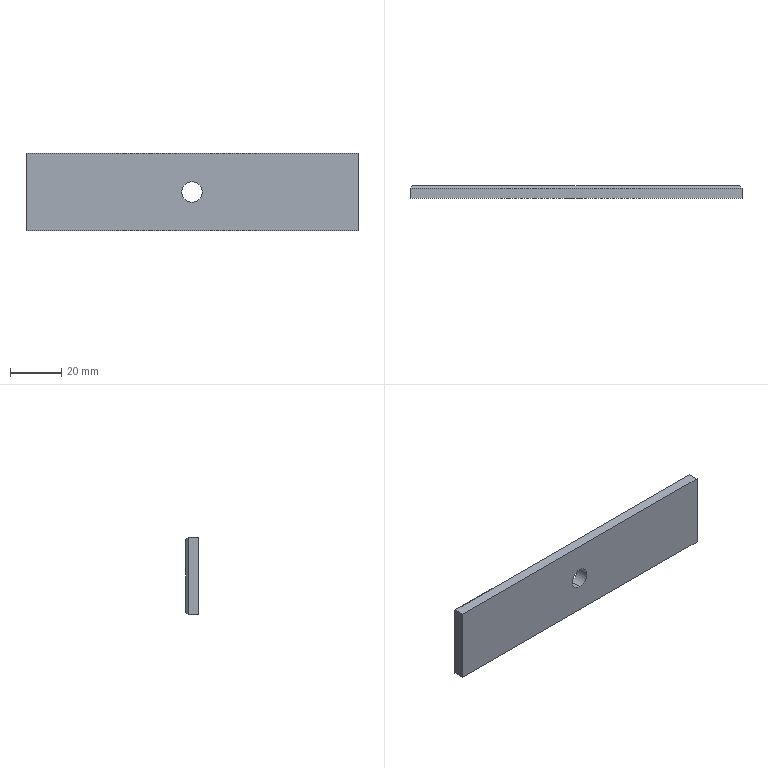Part | SolidWorks | features Chamfer 1, Cut 1, Extrusion 1 | 1 solid | 12 faces | box 129 x 5 x 30 mm | volume 18941 mm3 | plane 10 | cylinder 2 | commonest cylinder face diameters 8 x2
STEP:
#1=CARTESIAN_POINT('',(0.,0.,-4.));
#2=VERTEX_POINT('',#1);
#3=CARTESIAN_POINT('',(0.,0.,4.));
#4=VERTEX_POINT('',#3);
#5=CARTESIAN_POINT('',(0.,0.,0.));
#6=DIRECTION('',(0.,1.,0.));
#7=DIRECTION('',(0.,0.,-1.));
#8=AXIS2_PLACEMENT_3D('',#5,#6,#7);
#9=CIRCLE('',#8,4.);
#10=EDGE_CURVE('',#2,#4,#9,.T.);
#11=ORIENTED_EDGE('',*,*,#10,.F.);
#12=CARTESIAN_POINT('',(0.,5.,-4.));
#13=VERTEX_POINT('',#12);
#14=CARTESIAN_POINT('',(0.,-0.001,-4.));
#15=DIRECTION('',(0.,1.,0.));
#16=VECTOR('',#15,1000.);
#17=LINE('',#14,#16);
#18=EDGE_CURVE('',#2,#13,#17,.T.);
#19=ORIENTED_EDGE('',*,*,#18,.T.);
#20=CARTESIAN_POINT('',(0.,5.,4.));
#21=VERTEX_POINT('',#20);
#22=CARTESIAN_POINT('',(0.,5.,0.));
#23=DIRECTION('',(0.,1.,0.));
#24=DIRECTION('',(0.,0.,1.));
#25=AXIS2_PLACEMENT_3D('',#22,#23,#24);
#26=CIRCLE('',#25,4.);
#27=EDGE_CURVE('',#13,#21,#26,.T.);
#28=ORIENTED_EDGE('',*,*,#27,.T.);
#29=CARTESIAN_POINT('',(0.,-0.001,4.));
#30=DIRECTION('',(0.,1.,0.));
#31=VECTOR('',#30,1000.);
#32=LINE('',#29,#31);
#33=EDGE_CURVE('',#4,#21,#32,.T.);
#34=ORIENTED_EDGE('',*,*,#33,.F.);
#35=EDGE_LOOP('',(#11,#19,#28,#34));
#36=FACE_OUTER_BOUND('',#35,.T.);
#37=CARTESIAN_POINT('',(0.,-0.001,0.));
#38=DIRECTION('',(0.,1.,0.));
#39=DIRECTION('',(0.,0.,1.));
#40=AXIS2_PLACEMENT_3D('',#37,#38,#39);
#41=CYLINDRICAL_SURFACE('',#40,4.);
#42=ADVANCED_FACE('',(#36),#41,.F.);
#43=CARTESIAN_POINT('',(64.5,4.,-15.));
#44=VERTEX_POINT('',#43);
#45=CARTESIAN_POINT('',(64.5,0.,-15.));
#46=VERTEX_POINT('',#45);
#47=CARTESIAN_POINT('',(64.5,5.,-15.));
#48=DIRECTION('',(0.,-1.,0.));
#49=VECTOR('',#48,1000.);
#50=LINE('',#47,#49);
#51=EDGE_CURVE('',#44,#46,#50,.T.);
#52=ORIENTED_EDGE('',*,*,#51,.F.);
#53=CARTESIAN_POINT('',(64.5,4.,15.));
#54=VERTEX_POINT('',#53);
#55=CARTESIAN_POINT('',(64.5,4.,15.));
#56=DIRECTION('',(0.,0.,1.));
#57=VECTOR('',#56,1000.);
#58=LINE('',#55,#57);
#59=EDGE_CURVE('',#44,#54,#58,.T.);
#60=ORIENTED_EDGE('',*,*,#59,.T.);
#61=CARTESIAN_POINT('',(64.5,0.,15.));
#62=VERTEX_POINT('',#61);
#63=CARTESIAN_POINT('',(64.5,5.,15.));
#64=DIRECTION('',(0.,-1.,0.));
#65=VECTOR('',#64,1000.);
#66=LINE('',#63,#65);
#67=EDGE_CURVE('',#54,#62,#66,.T.);
#68=ORIENTED_EDGE('',*,*,#67,.T.);
#69=CARTESIAN_POINT('',(64.5,0.,15.));
#70=DIRECTION('',(0.,0.,-1.));
#71=VECTOR('',#70,1000.);
#72=LINE('',#69,#71);
#73=EDGE_CURVE('',#62,#46,#72,.T.);
#74=ORIENTED_EDGE('',*,*,#73,.T.);
#75=EDGE_LOOP('',(#52,#60,#68,#74));
#76=FACE_OUTER_BOUND('',#75,.T.);
#77=CARTESIAN_POINT('',(64.5,5.,15.));
#78=DIRECTION('',(-1.,0.,0.));
#79=DIRECTION('',(0.,0.,1.));
#80=AXIS2_PLACEMENT_3D('',#77,#78,#79);
#81=PLANE('',#80);
#82=ADVANCED_FACE('',(#76),#81,.F.);
#83=CARTESIAN_POINT('',(-64.5,4.,-15.));
#84=VERTEX_POINT('',#83);
#85=CARTESIAN_POINT('',(-64.5,0.,-15.));
#86=VERTEX_POINT('',#85);
#87=CARTESIAN_POINT('',(-64.5,5.,-15.));
#88=DIRECTION('',(0.,-1.,0.));
#89=VECTOR('',#88,1000.);
#90=LINE('',#87,#89);
#91=EDGE_CURVE('',#84,#86,#90,.T.);
#92=ORIENTED_EDGE('',*,*,#91,.F.);
#93=CARTESIAN_POINT('',(-64.5,4.,-15.));
#94=DIRECTION('',(1.,0.,0.));
#95=VECTOR('',#94,1000.);
#96=LINE('',#93,#95);
#97=EDGE_CURVE('',#84,#44,#96,.T.);
#98=ORIENTED_EDGE('',*,*,#97,.T.);
#99=ORIENTED_EDGE('',*,*,#51,.T.);
#100=CARTESIAN_POINT('',(-64.5,0.,-15.));
#101=DIRECTION('',(-1.,0.,0.));
#102=VECTOR('',#101,1000.);
#103=LINE('',#100,#102);
#104=EDGE_CURVE('',#46,#86,#103,.T.);
#105=ORIENTED_EDGE('',*,*,#104,.T.);
#106=EDGE_LOOP('',(#92,#98,#99,#105));
#107=FACE_OUTER_BOUND('',#106,.T.);
#108=CARTESIAN_POINT('',(-64.5,5.,-15.));
#109=DIRECTION('',(0.,0.,1.));
#110=DIRECTION('',(1.,0.,0.));
#111=AXIS2_PLACEMENT_3D('',#108,#109,#110);
#112=PLANE('',#111);
#113=ADVANCED_FACE('',(#107),#112,.F.);
#114=CARTESIAN_POINT('',(-64.5,4.,15.));
#115=VERTEX_POINT('',#114);
#116=CARTESIAN_POINT('',(-64.5,0.,15.));
#117=VERTEX_POINT('',#116);
#118=CARTESIAN_POINT('',(-64.5,5.,15.));
#119=DIRECTION('',(0.,-1.,0.));
#120=VECTOR('',#119,1000.);
#121=LINE('',#118,#120);
#122=EDGE_CURVE('',#115,#117,#121,.T.);
#123=ORIENTED_EDGE('',*,*,#122,.F.);
#124=CARTESIAN_POINT('',(-64.5,4.,15.));
#125=DIRECTION('',(0.,0.,-1.));
#126=VECTOR('',#125,1000.);
#127=LINE('',#124,#126);
#128=EDGE_CURVE('',#115,#84,#127,.T.);
#129=ORIENTED_EDGE('',*,*,#128,.T.);
#130=ORIENTED_EDGE('',*,*,#91,.T.);
#131=CARTESIAN_POINT('',(-64.5,0.,15.));
#132=DIRECTION('',(0.,0.,1.));
#133=VECTOR('',#132,1000.);
#134=LINE('',#131,#133);
#135=EDGE_CURVE('',#86,#117,#134,.T.);
#136=ORIENTED_EDGE('',*,*,#135,.T.);
#137=EDGE_LOOP('',(#123,#129,#130,#136));
#138=FACE_OUTER_BOUND('',#137,.T.);
#139=CARTESIAN_POINT('',(-64.5,5.,15.));
#140=DIRECTION('',(1.,0.,0.));
#141=DIRECTION('',(0.,0.,-1.));
#142=AXIS2_PLACEMENT_3D('',#139,#140,#141);
#143=PLANE('',#142);
#144=ADVANCED_FACE('',(#138),#143,.F.);
#145=ORIENTED_EDGE('',*,*,#67,.F.);
#146=CARTESIAN_POINT('',(-64.5,4.,15.));
#147=DIRECTION('',(-1.,0.,0.));
#148=VECTOR('',#147,1000.);
#149=LINE('',#146,#148);
#150=EDGE_CURVE('',#54,#115,#149,.T.);
#151=ORIENTED_EDGE('',*,*,#150,.T.);
#152=ORIENTED_EDGE('',*,*,#122,.T.);
#153=CARTESIAN_POINT('',(-64.5,0.,15.));
#154=DIRECTION('',(1.,0.,0.));
#155=VECTOR('',#154,1000.);
#156=LINE('',#153,#155);
#157=EDGE_CURVE('',#117,#62,#156,.T.);
#158=ORIENTED_EDGE('',*,*,#157,.T.);
#159=EDGE_LOOP('',(#145,#151,#152,#158));
#160=FACE_OUTER_BOUND('',#159,.T.);
#161=CARTESIAN_POINT('',(-64.5,5.,15.));
#162=DIRECTION('',(0.,0.,-1.));
#163=DIRECTION('',(-1.,0.,0.));
#164=AXIS2_PLACEMENT_3D('',#161,#162,#163);
#165=PLANE('',#164);
#166=ADVANCED_FACE('',(#160),#165,.F.);
#167=CARTESIAN_POINT('',(-63.5,5.,14.));
#168=VERTEX_POINT('',#167);
#169=CARTESIAN_POINT('',(63.5,5.,14.));
#170=VERTEX_POINT('',#169);
#171=CARTESIAN_POINT('',(0.,5.,14.));
#172=DIRECTION('',(1.,0.,0.));
#173=VECTOR('',#172,1000.);
#174=LINE('',#171,#173);
#175=EDGE_CURVE('',#168,#170,#174,.T.);
#176=ORIENTED_EDGE('',*,*,#175,.T.);
#177=CARTESIAN_POINT('',(63.5,5.,-14.));
#178=VERTEX_POINT('',#177);
#179=CARTESIAN_POINT('',(63.5,5.,0.));
#180=DIRECTION('',(0.,0.,-1.));
#181=VECTOR('',#180,1000.);
#182=LINE('',#179,#181);
#183=EDGE_CURVE('',#170,#178,#182,.T.);
#184=ORIENTED_EDGE('',*,*,#183,.T.);
#185=CARTESIAN_POINT('',(-63.5,5.,-14.));
#186=VERTEX_POINT('',#185);
#187=CARTESIAN_POINT('',(0.,5.,-14.));
#188=DIRECTION('',(-1.,0.,0.));
#189=VECTOR('',#188,1000.);
#190=LINE('',#187,#189);
#191=EDGE_CURVE('',#178,#186,#190,.T.);
#192=ORIENTED_EDGE('',*,*,#191,.T.);
#193=CARTESIAN_POINT('',(-63.5,5.,0.));
#194=DIRECTION('',(0.,0.,1.));
#195=VECTOR('',#194,1000.);
#196=LINE('',#193,#195);
#197=EDGE_CURVE('',#186,#168,#196,.T.);
#198=ORIENTED_EDGE('',*,*,#197,.T.);
#199=EDGE_LOOP('',(#176,#184,#192,#198));
#200=FACE_OUTER_BOUND('',#199,.T.);
#201=CARTESIAN_POINT('',(0.,5.,0.));
#202=DIRECTION('',(0.,1.,0.));
#203=DIRECTION('',(0.,0.,1.));
#204=AXIS2_PLACEMENT_3D('',#201,#202,#203);
#205=CIRCLE('',#204,4.);
#206=EDGE_CURVE('',#21,#13,#205,.T.);
#207=ORIENTED_EDGE('',*,*,#206,.F.);
#208=ORIENTED_EDGE('',*,*,#27,.F.);
#209=EDGE_LOOP('',(#207,#208));
#210=FACE_BOUND('',#209,.T.);
#211=CARTESIAN_POINT('',(0.,5.,0.));
#212=DIRECTION('',(0.,-1.,0.));
#213=DIRECTION('',(0.,0.,-1.));
#214=AXIS2_PLACEMENT_3D('',#211,#212,#213);
#215=PLANE('',#214);
#216=ADVANCED_FACE('',(#200,#210),#215,.F.);
#217=CARTESIAN_POINT('',(0.,0.,0.));
#218=DIRECTION('',(0.,1.,0.));
#219=DIRECTION('',(0.,0.,-1.));
#220=AXIS2_PLACEMENT_3D('',#217,#218,#219);
#221=CIRCLE('',#220,4.);
#222=EDGE_CURVE('',#4,#2,#221,.T.);
#223=ORIENTED_EDGE('',*,*,#222,.T.);
#224=ORIENTED_EDGE('',*,*,#10,.T.);
#225=EDGE_LOOP('',(#223,#224));
#226=FACE_BOUND('',#225,.T.);
#227=ORIENTED_EDGE('',*,*,#73,.F.);
#228=ORIENTED_EDGE('',*,*,#157,.F.);
#229=ORIENTED_EDGE('',*,*,#135,.F.);
#230=ORIENTED_EDGE('',*,*,#104,.F.);
#231=EDGE_LOOP('',(#227,#228,#229,#230));
#232=FACE_OUTER_BOUND('',#231,.T.);
#233=CARTESIAN_POINT('',(0.,0.,0.));
#234=DIRECTION('',(0.,-1.,0.));
#235=DIRECTION('',(0.,0.,-1.));
#236=AXIS2_PLACEMENT_3D('',#233,#234,#235);
#237=PLANE('',#236);
#238=ADVANCED_FACE('',(#226,#232),#237,.T.);
#239=ORIENTED_EDGE('',*,*,#18,.F.);
#240=ORIENTED_EDGE('',*,*,#222,.F.);
#241=ORIENTED_EDGE('',*,*,#33,.T.);
#242=ORIENTED_EDGE('',*,*,#206,.T.);
#243=EDGE_LOOP('',(#239,#240,#241,#242));
#244=FACE_OUTER_BOUND('',#243,.T.);
#245=CARTESIAN_POINT('',(0.,-0.001,0.));
#246=DIRECTION('',(0.,1.,0.));
#247=DIRECTION('',(0.,0.,1.));
#248=AXIS2_PLACEMENT_3D('',#245,#246,#247);
#249=CYLINDRICAL_SURFACE('',#248,4.);
#250=ADVANCED_FACE('',(#244),#249,.F.);
#251=CARTESIAN_POINT('',(-42.333,26.167,7.167));
#252=DIRECTION('',(0.5774,0.5774,0.5774));
#253=VECTOR('',#252,1000.);
#254=LINE('',#251,#253);
#255=EDGE_CURVE('',#84,#186,#254,.T.);
#256=ORIENTED_EDGE('',*,*,#255,.F.);
#257=ORIENTED_EDGE('',*,*,#128,.F.);
#258=CARTESIAN_POINT('',(-58.833,9.667,9.333));
#259=DIRECTION('',(-0.5774,-0.5774,0.5774));
#260=VECTOR('',#259,1000.);
#261=LINE('',#258,#260);
#262=EDGE_CURVE('',#168,#115,#261,.T.);
#263=ORIENTED_EDGE('',*,*,#262,.F.);
#264=ORIENTED_EDGE('',*,*,#197,.F.);
#265=EDGE_LOOP('',(#256,#257,#263,#264));
#266=FACE_OUTER_BOUND('',#265,.T.);
#267=CARTESIAN_POINT('',(-63.5,5.,0.));
#268=DIRECTION('',(0.7071,-0.7071,0.));
#269=DIRECTION('',(0.,0.,1.));
#270=AXIS2_PLACEMENT_3D('',#267,#268,#269);
#271=PLANE('',#270);
#272=ADVANCED_FACE('',(#266),#271,.F.);
#273=ORIENTED_EDGE('',*,*,#262,.T.);
#274=ORIENTED_EDGE('',*,*,#150,.F.);
#275=CARTESIAN_POINT('',(42.333,26.167,-7.167));
#276=DIRECTION('',(0.5774,-0.5774,0.5774));
#277=VECTOR('',#276,1000.);
#278=LINE('',#275,#277);
#279=EDGE_CURVE('',#170,#54,#278,.T.);
#280=ORIENTED_EDGE('',*,*,#279,.F.);
#281=ORIENTED_EDGE('',*,*,#175,.F.);
#282=EDGE_LOOP('',(#273,#274,#280,#281));
#283=FACE_OUTER_BOUND('',#282,.T.);
#284=CARTESIAN_POINT('',(0.,5.,14.));
#285=DIRECTION('',(0.,-0.7071,-0.7071));
#286=DIRECTION('',(1.,0.,0.));
#287=AXIS2_PLACEMENT_3D('',#284,#285,#286);
#288=PLANE('',#287);
#289=ADVANCED_FACE('',(#283),#288,.F.);
#290=ORIENTED_EDGE('',*,*,#255,.T.);
#291=ORIENTED_EDGE('',*,*,#191,.F.);
#292=CARTESIAN_POINT('',(42.333,26.167,7.167));
#293=DIRECTION('',(-0.5774,0.5774,0.5774));
#294=VECTOR('',#293,1000.);
#295=LINE('',#292,#294);
#296=EDGE_CURVE('',#44,#178,#295,.T.);
#297=ORIENTED_EDGE('',*,*,#296,.F.);
#298=ORIENTED_EDGE('',*,*,#97,.F.);
#299=EDGE_LOOP('',(#290,#291,#297,#298));
#300=FACE_OUTER_BOUND('',#299,.T.);
#301=CARTESIAN_POINT('',(0.,5.,-14.));
#302=DIRECTION('',(0.,-0.7071,0.7071));
#303=DIRECTION('',(-1.,0.,0.));
#304=AXIS2_PLACEMENT_3D('',#301,#302,#303);
#305=PLANE('',#304);
#306=ADVANCED_FACE('',(#300),#305,.F.);
#307=ORIENTED_EDGE('',*,*,#279,.T.);
#308=ORIENTED_EDGE('',*,*,#59,.F.);
#309=ORIENTED_EDGE('',*,*,#296,.T.);
#310=ORIENTED_EDGE('',*,*,#183,.F.);
#311=EDGE_LOOP('',(#307,#308,#309,#310));
#312=FACE_OUTER_BOUND('',#311,.T.);
#313=CARTESIAN_POINT('',(63.5,5.,0.));
#314=DIRECTION('',(-0.7071,-0.7071,0.));
#315=DIRECTION('',(0.,0.,-1.));
#316=AXIS2_PLACEMENT_3D('',#313,#314,#315);
#317=PLANE('',#316);
#318=ADVANCED_FACE('',(#312),#317,.F.);
#319=CLOSED_SHELL('',(#42,#82,#113,#144,#166,#216,#238,#250,#272,#289,#306,#318));
#320=MANIFOLD_SOLID_BREP('',#319);
#321=CARTESIAN_POINT('',(0.,0.,0.));
#322=DIRECTION('',(0.,0.,1.));
#323=DIRECTION('',(1.,0.,0.));
#324=AXIS2_PLACEMENT_3D('',#321,#322,#323);
#325=(LENGTH_UNIT()NAMED_UNIT(*)SI_UNIT(.MILLI.,.METRE.));
#326=UNCERTAINTY_MEASURE_WITH_UNIT(LENGTH_MEASURE(0.00001),#325,'','');
#327=(NAMED_UNIT(*)PLANE_ANGLE_UNIT()SI_UNIT($,.RADIAN.));
#328=(NAMED_UNIT(*)SI_UNIT($,.STERADIAN.)SOLID_ANGLE_UNIT());
#329=(GEOMETRIC_REPRESENTATION_CONTEXT(3)GLOBAL_UNCERTAINTY_ASSIGNED_CONTEXT((#326))GLOBAL_UNIT_ASSIGNED_CONTEXT((#325,#327,#328))REPRESENTATION_CONTEXT('',''));
#330=ADVANCED_BREP_SHAPE_REPRESENTATION('',(#320,#324),#329);